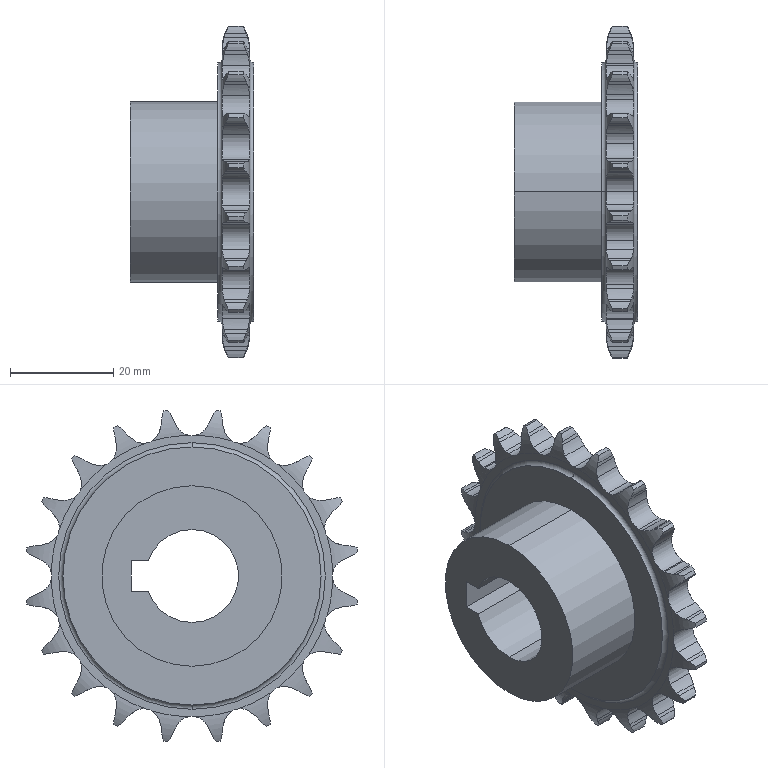Part | STEP file | Drive sprocket_05B | 1 solid | 230 faces | box 24 x 64.324 x 64.324 mm | volume 27131 mm3 | cylinder 138 | plane 48 | torus 44 | commonest cylinder face diameters 9.196 x42 16.642 x42 6.482 x25 65 x20 50 x4 18 x3